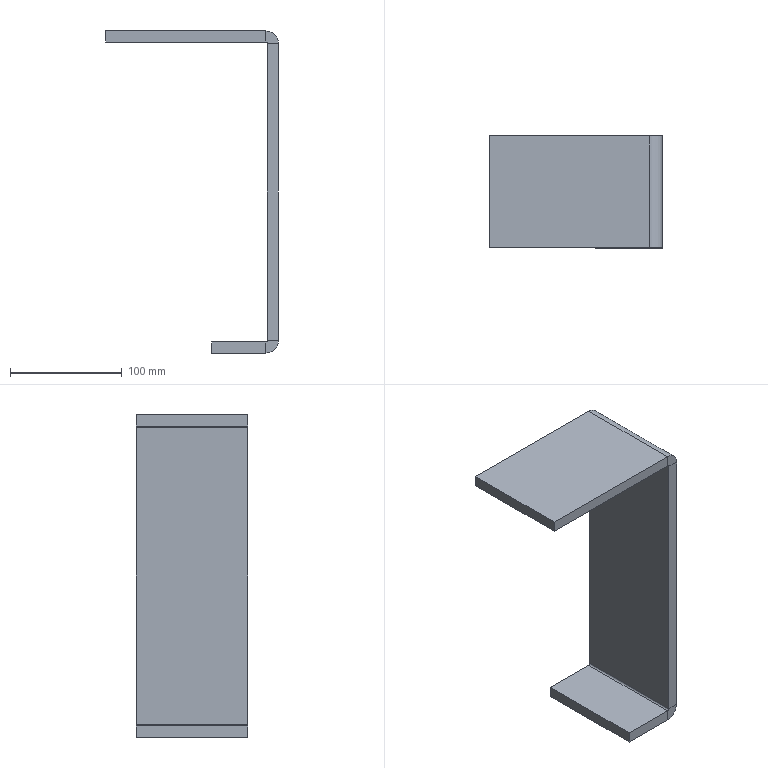Part | STEP file | A1 | 1 solid | 22 faces | box 155 x 100 x 289 mm | volume 478420 mm3 | plane 18 | cylinder 4 | commonest cylinder face diameters 3 x2 23 x2
STEP:
#1=CARTESIAN_POINT('',(0.,0.,0.));
#2=DIRECTION('',(0.,0.,1.));
#3=DIRECTION('',(1.,0.,0.));
#4=AXIS2_PLACEMENT_3D('',#1,#2,#3);
#5=CARTESIAN_POINT('',(50.,100.,267.5));
#6=VERTEX_POINT('',#5);
#7=CARTESIAN_POINT('',(60.,100.,267.5));
#8=VERTEX_POINT('',#7);
#9=CARTESIAN_POINT('',(50.,100.,267.5));
#10=DIRECTION('',(1.,0.,0.));
#11=VECTOR('',#10,1.);
#12=LINE('',#9,#11);
#13=CARTESIAN_POINT('',(60.,100.,279.));
#14=DIRECTION('',(0.,-1.,0.));
#15=DIRECTION('',(1.,0.,0.));
#16=AXIS2_PLACEMENT_3D('',#13,#14,#15);
#17=PLANE('',#16);
#18=CARTESIAN_POINT('',(-10.,-11.5));
#19=DIRECTION('',(1.,0.));
#20=VECTOR('',#19,1.);
#21=LINE('',#18,#20);
#22=(GEOMETRIC_REPRESENTATION_CONTEXT(2)PARAMETRIC_REPRESENTATION_CONTEXT()REPRESENTATION_CONTEXT('',''));
#23=DEFINITIONAL_REPRESENTATION('',(#21),#22);
#24=PCURVE('',#17,#23);
#25=CARTESIAN_POINT('',(48.5,100.,267.5));
#26=DIRECTION('',(0.,-1.,0.));
#27=DIRECTION('',(0.,0.,-1.));
#28=AXIS2_PLACEMENT_3D('',#25,#26,#27);
#29=PLANE('',#28);
#30=CARTESIAN_POINT('',(0.,1.5));
#31=DIRECTION('',(0.,1.));
#32=VECTOR('',#31,1.);
#33=LINE('',#30,#32);
#34=(GEOMETRIC_REPRESENTATION_CONTEXT(2)PARAMETRIC_REPRESENTATION_CONTEXT()REPRESENTATION_CONTEXT('',''));
#35=DEFINITIONAL_REPRESENTATION('',(#33),#34);
#36=PCURVE('',#29,#35);
#37=SURFACE_CURVE('',#12,(#24,#36),.PCURVE_S1.);
#38=EDGE_CURVE('',#6,#8,#37,.T.);
#39=ORIENTED_EDGE('',*,*,#38,.T.);
#40=CARTESIAN_POINT('',(60.,100.,1.5));
#41=VERTEX_POINT('',#40);
#42=CARTESIAN_POINT('',(60.,100.,0.));
#43=DIRECTION('',(0.,0.,1.));
#44=VECTOR('',#43,1.);
#45=LINE('',#42,#44);
#46=CARTESIAN_POINT('',(0.,-279.));
#47=DIRECTION('',(0.,1.));
#48=VECTOR('',#47,1.);
#49=LINE('',#46,#48);
#50=(GEOMETRIC_REPRESENTATION_CONTEXT(2)PARAMETRIC_REPRESENTATION_CONTEXT()REPRESENTATION_CONTEXT('',''));
#51=DEFINITIONAL_REPRESENTATION('',(#49),#50);
#52=PCURVE('',#17,#51);
#53=CARTESIAN_POINT('',(60.,0.,0.));
#54=DIRECTION('',(-1.,0.,0.));
#55=DIRECTION('',(0.,0.,1.));
#56=AXIS2_PLACEMENT_3D('',#53,#54,#55);
#57=PLANE('',#56);
#58=CARTESIAN_POINT('',(0.,100.));
#59=DIRECTION('',(1.,0.));
#60=VECTOR('',#59,1.);
#61=LINE('',#58,#60);
#62=(GEOMETRIC_REPRESENTATION_CONTEXT(2)PARAMETRIC_REPRESENTATION_CONTEXT()REPRESENTATION_CONTEXT('',''));
#63=DEFINITIONAL_REPRESENTATION('',(#61),#62);
#64=PCURVE('',#57,#63);
#65=SURFACE_CURVE('',#45,(#52,#64),.PCURVE_S1.);
#66=EDGE_CURVE('',#41,#8,#65,.T.);
#67=ORIENTED_EDGE('',*,*,#66,.F.);
#68=CARTESIAN_POINT('',(50.,100.,1.5));
#69=VERTEX_POINT('',#68);
#70=CARTESIAN_POINT('',(50.,100.,1.5));
#71=DIRECTION('',(1.,0.,0.));
#72=VECTOR('',#71,1.);
#73=LINE('',#70,#72);
#74=CARTESIAN_POINT('',(-10.,-277.5));
#75=DIRECTION('',(1.,0.));
#76=VECTOR('',#75,1.);
#77=LINE('',#74,#76);
#78=(GEOMETRIC_REPRESENTATION_CONTEXT(2)PARAMETRIC_REPRESENTATION_CONTEXT()REPRESENTATION_CONTEXT('',''));
#79=DEFINITIONAL_REPRESENTATION('',(#77),#78);
#80=PCURVE('',#17,#79);
#81=CARTESIAN_POINT('',(48.5,100.,1.5));
#82=DIRECTION('',(0.,-1.,0.));
#83=DIRECTION('',(0.,0.,-1.));
#84=AXIS2_PLACEMENT_3D('',#81,#82,#83);
#85=PLANE('',#84);
#86=CARTESIAN_POINT('',(0.,1.5));
#87=DIRECTION('',(0.,1.));
#88=VECTOR('',#87,1.);
#89=LINE('',#86,#88);
#90=(GEOMETRIC_REPRESENTATION_CONTEXT(2)PARAMETRIC_REPRESENTATION_CONTEXT()REPRESENTATION_CONTEXT('',''));
#91=DEFINITIONAL_REPRESENTATION('',(#89),#90);
#92=PCURVE('',#85,#91);
#93=SURFACE_CURVE('',#73,(#80,#92),.PCURVE_S1.);
#94=EDGE_CURVE('',#69,#41,#93,.T.);
#95=ORIENTED_EDGE('',*,*,#94,.F.);
#96=CARTESIAN_POINT('',(50.,100.,279.));
#97=DIRECTION('',(0.,0.,1.));
#98=VECTOR('',#97,1.);
#99=LINE('',#96,#98);
#100=CARTESIAN_POINT('',(-10.,0.));
#101=DIRECTION('',(0.,1.));
#102=VECTOR('',#101,1.);
#103=LINE('',#100,#102);
#104=(GEOMETRIC_REPRESENTATION_CONTEXT(2)PARAMETRIC_REPRESENTATION_CONTEXT()REPRESENTATION_CONTEXT('',''));
#105=DEFINITIONAL_REPRESENTATION('',(#103),#104);
#106=PCURVE('',#17,#105);
#107=CARTESIAN_POINT('',(50.,0.,0.));
#108=DIRECTION('',(-1.,0.,0.));
#109=DIRECTION('',(0.,0.,1.));
#110=AXIS2_PLACEMENT_3D('',#107,#108,#109);
#111=PLANE('',#110);
#112=CARTESIAN_POINT('',(279.,100.));
#113=DIRECTION('',(1.,0.));
#114=VECTOR('',#113,1.);
#115=LINE('',#112,#114);
#116=(GEOMETRIC_REPRESENTATION_CONTEXT(2)PARAMETRIC_REPRESENTATION_CONTEXT()REPRESENTATION_CONTEXT('',''));
#117=DEFINITIONAL_REPRESENTATION('',(#115),#116);
#118=PCURVE('',#111,#117);
#119=SURFACE_CURVE('',#99,(#106,#118),.PCURVE_S1.);
#120=EDGE_CURVE('',#69,#6,#119,.T.);
#121=ORIENTED_EDGE('',*,*,#120,.T.);
#122=EDGE_LOOP('',(#39,#67,#95,#121));
#123=FACE_BOUND('',#122,.T.);
#124=ADVANCED_FACE('',(#123),#17,.F.);
#125=CARTESIAN_POINT('',(50.,0.,267.5));
#126=VERTEX_POINT('',#125);
#127=CARTESIAN_POINT('',(60.,0.,267.5));
#128=VERTEX_POINT('',#127);
#129=CARTESIAN_POINT('',(50.,0.,267.5));
#130=DIRECTION('',(1.,0.,0.));
#131=VECTOR('',#130,1.);
#132=LINE('',#129,#131);
#133=CARTESIAN_POINT('',(60.,0.,0.));
#134=DIRECTION('',(0.,1.,0.));
#135=DIRECTION('',(-1.,0.,0.));
#136=AXIS2_PLACEMENT_3D('',#133,#134,#135);
#137=PLANE('',#136);
#138=CARTESIAN_POINT('',(10.,267.5));
#139=DIRECTION('',(-1.,0.));
#140=VECTOR('',#139,1.);
#141=LINE('',#138,#140);
#142=(GEOMETRIC_REPRESENTATION_CONTEXT(2)PARAMETRIC_REPRESENTATION_CONTEXT()REPRESENTATION_CONTEXT('',''));
#143=DEFINITIONAL_REPRESENTATION('',(#141),#142);
#144=PCURVE('',#137,#143);
#145=CARTESIAN_POINT('',(48.5,0.,267.5));
#146=DIRECTION('',(0.,-1.,0.));
#147=DIRECTION('',(0.,0.,-1.));
#148=AXIS2_PLACEMENT_3D('',#145,#146,#147);
#149=PLANE('',#148);
#150=CARTESIAN_POINT('',(0.,1.5));
#151=DIRECTION('',(0.,1.));
#152=VECTOR('',#151,1.);
#153=LINE('',#150,#152);
#154=(GEOMETRIC_REPRESENTATION_CONTEXT(2)PARAMETRIC_REPRESENTATION_CONTEXT()REPRESENTATION_CONTEXT('',''));
#155=DEFINITIONAL_REPRESENTATION('',(#153),#154);
#156=PCURVE('',#149,#155);
#157=SURFACE_CURVE('',#132,(#144,#156),.PCURVE_S1.);
#158=EDGE_CURVE('',#126,#128,#157,.T.);
#159=ORIENTED_EDGE('',*,*,#158,.F.);
#160=CARTESIAN_POINT('',(50.,0.,1.5));
#161=VERTEX_POINT('',#160);
#162=CARTESIAN_POINT('',(50.,0.,0.));
#163=DIRECTION('',(0.,0.,-1.));
#164=VECTOR('',#163,1.);
#165=LINE('',#162,#164);
#166=CARTESIAN_POINT('',(10.,0.));
#167=DIRECTION('',(0.,-1.));
#168=VECTOR('',#167,1.);
#169=LINE('',#166,#168);
#170=(GEOMETRIC_REPRESENTATION_CONTEXT(2)PARAMETRIC_REPRESENTATION_CONTEXT()REPRESENTATION_CONTEXT('',''));
#171=DEFINITIONAL_REPRESENTATION('',(#169),#170);
#172=PCURVE('',#137,#171);
#173=CARTESIAN_POINT('',(0.,0.));
#174=DIRECTION('',(-1.,0.));
#175=VECTOR('',#174,1.);
#176=LINE('',#173,#175);
#177=(GEOMETRIC_REPRESENTATION_CONTEXT(2)PARAMETRIC_REPRESENTATION_CONTEXT()REPRESENTATION_CONTEXT('',''));
#178=DEFINITIONAL_REPRESENTATION('',(#176),#177);
#179=PCURVE('',#111,#178);
#180=SURFACE_CURVE('',#165,(#172,#179),.PCURVE_S1.);
#181=EDGE_CURVE('',#126,#161,#180,.T.);
#182=ORIENTED_EDGE('',*,*,#181,.T.);
#183=CARTESIAN_POINT('',(60.,0.,1.5));
#184=VERTEX_POINT('',#183);
#185=CARTESIAN_POINT('',(60.,0.,1.5));
#186=DIRECTION('',(1.,0.,0.));
#187=VECTOR('',#186,1.);
#188=LINE('',#185,#187);
#189=CARTESIAN_POINT('',(0.,1.5));
#190=DIRECTION('',(-1.,0.));
#191=VECTOR('',#190,1.);
#192=LINE('',#189,#191);
#193=(GEOMETRIC_REPRESENTATION_CONTEXT(2)PARAMETRIC_REPRESENTATION_CONTEXT()REPRESENTATION_CONTEXT('',''));
#194=DEFINITIONAL_REPRESENTATION('',(#192),#193);
#195=PCURVE('',#137,#194);
#196=CARTESIAN_POINT('',(48.5,0.,1.5));
#197=DIRECTION('',(0.,-1.,0.));
#198=DIRECTION('',(0.,0.,-1.));
#199=AXIS2_PLACEMENT_3D('',#196,#197,#198);
#200=PLANE('',#199);
#201=CARTESIAN_POINT('',(0.,11.5));
#202=DIRECTION('',(0.,1.));
#203=VECTOR('',#202,1.);
#204=LINE('',#201,#203);
#205=(GEOMETRIC_REPRESENTATION_CONTEXT(2)PARAMETRIC_REPRESENTATION_CONTEXT()REPRESENTATION_CONTEXT('',''));
#206=DEFINITIONAL_REPRESENTATION('',(#204),#205);
#207=PCURVE('',#200,#206);
#208=SURFACE_CURVE('',#188,(#195,#207),.PCURVE_S1.);
#209=EDGE_CURVE('',#161,#184,#208,.T.);
#210=ORIENTED_EDGE('',*,*,#209,.T.);
#211=CARTESIAN_POINT('',(60.,0.,0.));
#212=DIRECTION('',(0.,0.,-1.));
#213=VECTOR('',#212,1.);
#214=LINE('',#211,#213);
#215=CARTESIAN_POINT('',(0.,0.));
#216=DIRECTION('',(0.,-1.));
#217=VECTOR('',#216,1.);
#218=LINE('',#215,#217);
#219=(GEOMETRIC_REPRESENTATION_CONTEXT(2)PARAMETRIC_REPRESENTATION_CONTEXT()REPRESENTATION_CONTEXT('',''));
#220=DEFINITIONAL_REPRESENTATION('',(#218),#219);
#221=PCURVE('',#137,#220);
#222=CARTESIAN_POINT('',(0.,0.));
#223=DIRECTION('',(-1.,0.));
#224=VECTOR('',#223,1.);
#225=LINE('',#222,#224);
#226=(GEOMETRIC_REPRESENTATION_CONTEXT(2)PARAMETRIC_REPRESENTATION_CONTEXT()REPRESENTATION_CONTEXT('',''));
#227=DEFINITIONAL_REPRESENTATION('',(#225),#226);
#228=PCURVE('',#57,#227);
#229=SURFACE_CURVE('',#214,(#221,#228),.PCURVE_S1.);
#230=EDGE_CURVE('',#128,#184,#229,.T.);
#231=ORIENTED_EDGE('',*,*,#230,.F.);
#232=EDGE_LOOP('',(#159,#182,#210,#231));
#233=FACE_BOUND('',#232,.T.);
#234=ADVANCED_FACE('',(#233),#137,.F.);
#235=CARTESIAN_POINT('',(60.,100.,267.5));
#236=DIRECTION('',(0.,-1.,0.));
#237=VECTOR('',#236,1.);
#238=LINE('',#235,#237);
#239=CARTESIAN_POINT('',(267.5,100.));
#240=DIRECTION('',(0.,-1.));
#241=VECTOR('',#240,1.);
#242=LINE('',#239,#241);
#243=(GEOMETRIC_REPRESENTATION_CONTEXT(2)PARAMETRIC_REPRESENTATION_CONTEXT()REPRESENTATION_CONTEXT('',''));
#244=DEFINITIONAL_REPRESENTATION('',(#242),#243);
#245=PCURVE('',#57,#244);
#246=CARTESIAN_POINT('',(48.5,100.,267.5));
#247=DIRECTION('',(0.,1.,0.));
#248=DIRECTION('',(0.,0.,1.));
#249=AXIS2_PLACEMENT_3D('',#246,#247,#248);
#250=CYLINDRICAL_SURFACE('',#249,11.5);
#251=CARTESIAN_POINT('',(1.571,0.));
#252=DIRECTION('',(0.,-1.));
#253=VECTOR('',#252,1.);
#254=LINE('',#251,#253);
#255=(GEOMETRIC_REPRESENTATION_CONTEXT(2)PARAMETRIC_REPRESENTATION_CONTEXT()REPRESENTATION_CONTEXT('',''));
#256=DEFINITIONAL_REPRESENTATION('',(#254),#255);
#257=PCURVE('',#250,#256);
#258=SURFACE_CURVE('',#238,(#245,#257),.PCURVE_S1.);
#259=EDGE_CURVE('',#8,#128,#258,.T.);
#260=ORIENTED_EDGE('',*,*,#259,.T.);
#261=ORIENTED_EDGE('',*,*,#230,.T.);
#262=CARTESIAN_POINT('',(60.,0.,1.5));
#263=DIRECTION('',(0.,-1.,0.));
#264=VECTOR('',#263,1.);
#265=LINE('',#262,#264);
#266=CARTESIAN_POINT('',(1.5,0.));
#267=DIRECTION('',(0.,-1.));
#268=VECTOR('',#267,1.);
#269=LINE('',#266,#268);
#270=(GEOMETRIC_REPRESENTATION_CONTEXT(2)PARAMETRIC_REPRESENTATION_CONTEXT()REPRESENTATION_CONTEXT('',''));
#271=DEFINITIONAL_REPRESENTATION('',(#269),#270);
#272=PCURVE('',#57,#271);
#273=CARTESIAN_POINT('',(48.5,100.,1.5));
#274=DIRECTION('',(0.,1.,0.));
#275=DIRECTION('',(1.,0.,0.));
#276=AXIS2_PLACEMENT_3D('',#273,#274,#275);
#277=CYLINDRICAL_SURFACE('',#276,11.5);
#278=CARTESIAN_POINT('',(0.,-100.));
#279=DIRECTION('',(0.,-1.));
#280=VECTOR('',#279,1.);
#281=LINE('',#278,#280);
#282=(GEOMETRIC_REPRESENTATION_CONTEXT(2)PARAMETRIC_REPRESENTATION_CONTEXT()REPRESENTATION_CONTEXT('',''));
#283=DEFINITIONAL_REPRESENTATION('',(#281),#282);
#284=PCURVE('',#277,#283);
#285=SURFACE_CURVE('',#265,(#272,#284),.PCURVE_S1.);
#286=EDGE_CURVE('',#41,#184,#285,.T.);
#287=ORIENTED_EDGE('',*,*,#286,.F.);
#288=ORIENTED_EDGE('',*,*,#66,.T.);
#289=EDGE_LOOP('',(#260,#261,#287,#288));
#290=FACE_BOUND('',#289,.T.);
#291=ADVANCED_FACE('',(#290),#57,.F.);
#292=ORIENTED_EDGE('',*,*,#181,.F.);
#293=CARTESIAN_POINT('',(50.,100.,267.5));
#294=DIRECTION('',(0.,-1.,0.));
#295=VECTOR('',#294,1.);
#296=LINE('',#293,#295);
#297=CARTESIAN_POINT('',(267.5,100.));
#298=DIRECTION('',(0.,-1.));
#299=VECTOR('',#298,1.);
#300=LINE('',#297,#299);
#301=(GEOMETRIC_REPRESENTATION_CONTEXT(2)PARAMETRIC_REPRESENTATION_CONTEXT()REPRESENTATION_CONTEXT('',''));
#302=DEFINITIONAL_REPRESENTATION('',(#300),#301);
#303=PCURVE('',#111,#302);
#304=CARTESIAN_POINT('',(48.5,100.,267.5));
#305=DIRECTION('',(0.,1.,0.));
#306=DIRECTION('',(0.,0.,1.));
#307=AXIS2_PLACEMENT_3D('',#304,#305,#306);
#308=CYLINDRICAL_SURFACE('',#307,1.5);
#309=CARTESIAN_POINT('',(1.571,0.));
#310=DIRECTION('',(0.,-1.));
#311=VECTOR('',#310,1.);
#312=LINE('',#309,#311);
#313=(GEOMETRIC_REPRESENTATION_CONTEXT(2)PARAMETRIC_REPRESENTATION_CONTEXT()REPRESENTATION_CONTEXT('',''));
#314=DEFINITIONAL_REPRESENTATION('',(#312),#313);
#315=PCURVE('',#308,#314);
#316=SURFACE_CURVE('',#296,(#303,#315),.PCURVE_S1.);
#317=EDGE_CURVE('',#6,#126,#316,.T.);
#318=ORIENTED_EDGE('',*,*,#317,.F.);
#319=ORIENTED_EDGE('',*,*,#120,.F.);
#320=CARTESIAN_POINT('',(50.,0.,1.5));
#321=DIRECTION('',(0.,1.,0.));
#322=VECTOR('',#321,1.);
#323=LINE('',#320,#322);
#324=CARTESIAN_POINT('',(1.5,0.));
#325=DIRECTION('',(0.,1.));
#326=VECTOR('',#325,1.);
#327=LINE('',#324,#326);
#328=(GEOMETRIC_REPRESENTATION_CONTEXT(2)PARAMETRIC_REPRESENTATION_CONTEXT()REPRESENTATION_CONTEXT('',''));
#329=DEFINITIONAL_REPRESENTATION('',(#327),#328);
#330=PCURVE('',#111,#329);
#331=CARTESIAN_POINT('',(48.5,100.,1.5));
#332=DIRECTION('',(0.,1.,0.));
#333=DIRECTION('',(1.,0.,0.));
#334=AXIS2_PLACEMENT_3D('',#331,#332,#333);
#335=CYLINDRICAL_SURFACE('',#334,1.5);
#336=CARTESIAN_POINT('',(0.,-100.));
#337=DIRECTION('',(0.,1.));
#338=VECTOR('',#337,1.);
#339=LINE('',#336,#338);
#340=(GEOMETRIC_REPRESENTATION_CONTEXT(2)PARAMETRIC_REPRESENTATION_CONTEXT()REPRESENTATION_CONTEXT('',''));
#341=DEFINITIONAL_REPRESENTATION('',(#339),#340);
#342=PCURVE('',#335,#341);
#343=SURFACE_CURVE('',#323,(#330,#342),.PCURVE_S1.);
#344=EDGE_CURVE('',#161,#69,#343,.T.);
#345=ORIENTED_EDGE('',*,*,#344,.F.);
#346=EDGE_LOOP('',(#292,#318,#319,#345));
#347=FACE_BOUND('',#346,.T.);
#348=ADVANCED_FACE('',(#347),#111,.T.);
#349=CARTESIAN_POINT('',(48.5,100.,0.));
#350=VERTEX_POINT('',#349);
#351=CARTESIAN_POINT('',(0.,100.,0.));
#352=VERTEX_POINT('',#351);
#353=CARTESIAN_POINT('',(0.,100.,0.));
#354=DIRECTION('',(-1.,0.,0.));
#355=VECTOR('',#354,1.);
#356=LINE('',#353,#355);
#357=CARTESIAN_POINT('',(0.,100.,-10.));
#358=DIRECTION('',(0.,1.,0.));
#359=DIRECTION('',(-1.,0.,0.));
#360=AXIS2_PLACEMENT_3D('',#357,#358,#359);
#361=PLANE('',#360);
#362=CARTESIAN_POINT('',(0.,10.));
#363=DIRECTION('',(1.,0.));
#364=VECTOR('',#363,1.);
#365=LINE('',#362,#364);
#366=(GEOMETRIC_REPRESENTATION_CONTEXT(2)PARAMETRIC_REPRESENTATION_CONTEXT()REPRESENTATION_CONTEXT('',''));
#367=DEFINITIONAL_REPRESENTATION('',(#365),#366);
#368=PCURVE('',#361,#367);
#369=CARTESIAN_POINT('',(0.,0.,0.));
#370=DIRECTION('',(0.,0.,1.));
#371=DIRECTION('',(1.,0.,0.));
#372=AXIS2_PLACEMENT_3D('',#369,#370,#371);
#373=PLANE('',#372);
#374=CARTESIAN_POINT('',(0.,100.));
#375=DIRECTION('',(-1.,0.));
#376=VECTOR('',#375,1.);
#377=LINE('',#374,#376);
#378=(GEOMETRIC_REPRESENTATION_CONTEXT(2)PARAMETRIC_REPRESENTATION_CONTEXT()REPRESENTATION_CONTEXT('',''));
#379=DEFINITIONAL_REPRESENTATION('',(#377),#378);
#380=PCURVE('',#373,#379);
#381=SURFACE_CURVE('',#356,(#368,#380),.PCURVE_S1.);
#382=EDGE_CURVE('',#350,#352,#381,.T.);
#383=ORIENTED_EDGE('',*,*,#382,.F.);
#384=CARTESIAN_POINT('',(48.5,100.,-10.));
#385=VERTEX_POINT('',#384);
#386=CARTESIAN_POINT('',(48.5,100.,0.));
#387=DIRECTION('',(0.,0.,-1.));
#388=VECTOR('',#387,1.);
#389=LINE('',#386,#388);
#390=CARTESIAN_POINT('',(-48.5,10.));
#391=DIRECTION('',(0.,-1.));
#392=VECTOR('',#391,1.);
#393=LINE('',#390,#392);
#394=(GEOMETRIC_REPRESENTATION_CONTEXT(2)PARAMETRIC_REPRESENTATION_CONTEXT()REPRESENTATION_CONTEXT('',''));
#395=DEFINITIONAL_REPRESENTATION('',(#393),#394);
#396=PCURVE('',#361,#395);
#397=CARTESIAN_POINT('',(1.5,0.));
#398=DIRECTION('',(1.,0.));
#399=VECTOR('',#398,1.);
#400=LINE('',#397,#399);
#401=(GEOMETRIC_REPRESENTATION_CONTEXT(2)PARAMETRIC_REPRESENTATION_CONTEXT()REPRESENTATION_CONTEXT('',''));
#402=DEFINITIONAL_REPRESENTATION('',(#400),#401);
#403=PCURVE('',#85,#402);
#404=SURFACE_CURVE('',#389,(#396,#403),.PCURVE_S1.);
#405=EDGE_CURVE('',#350,#385,#404,.T.);
#406=ORIENTED_EDGE('',*,*,#405,.T.);
#407=CARTESIAN_POINT('',(0.,100.,-10.));
#408=VERTEX_POINT('',#407);
#409=CARTESIAN_POINT('',(0.,100.,-10.));
#410=DIRECTION('',(-1.,0.,0.));
#411=VECTOR('',#410,1.);
#412=LINE('',#409,#411);
#413=CARTESIAN_POINT('',(0.,0.));
#414=DIRECTION('',(1.,0.));
#415=VECTOR('',#414,1.);
#416=LINE('',#413,#415);
#417=(GEOMETRIC_REPRESENTATION_CONTEXT(2)PARAMETRIC_REPRESENTATION_CONTEXT()REPRESENTATION_CONTEXT('',''));
#418=DEFINITIONAL_REPRESENTATION('',(#416),#417);
#419=PCURVE('',#361,#418);
#420=CARTESIAN_POINT('',(0.,0.,-10.));
#421=DIRECTION('',(0.,0.,1.));
#422=DIRECTION('',(1.,0.,0.));
#423=AXIS2_PLACEMENT_3D('',#420,#421,#422);
#424=PLANE('',#423);
#425=CARTESIAN_POINT('',(0.,100.));
#426=DIRECTION('',(-1.,0.));
#427=VECTOR('',#426,1.);
#428=LINE('',#425,#427);
#429=(GEOMETRIC_REPRESENTATION_CONTEXT(2)PARAMETRIC_REPRESENTATION_CONTEXT()REPRESENTATION_CONTEXT('',''));
#430=DEFINITIONAL_REPRESENTATION('',(#428),#429);
#431=PCURVE('',#424,#430);
#432=SURFACE_CURVE('',#412,(#419,#431),.PCURVE_S1.);
#433=EDGE_CURVE('',#385,#408,#432,.T.);
#434=ORIENTED_EDGE('',*,*,#433,.T.);
#435=CARTESIAN_POINT('',(0.,100.,-10.));
#436=DIRECTION('',(0.,0.,1.));
#437=VECTOR('',#436,1.);
#438=LINE('',#435,#437);
#439=CARTESIAN_POINT('',(0.,0.));
#440=DIRECTION('',(0.,1.));
#441=VECTOR('',#440,1.);
#442=LINE('',#439,#441);
#443=(GEOMETRIC_REPRESENTATION_CONTEXT(2)PARAMETRIC_REPRESENTATION_CONTEXT()REPRESENTATION_CONTEXT('',''));
#444=DEFINITIONAL_REPRESENTATION('',(#442),#443);
#445=PCURVE('',#361,#444);
#446=CARTESIAN_POINT('',(0.,100.,-10.));
#447=DIRECTION('',(-1.,0.,0.));
#448=DIRECTION('',(0.,-1.,0.));
#449=AXIS2_PLACEMENT_3D('',#446,#447,#448);
#450=PLANE('',#449);
#451=CARTESIAN_POINT('',(0.,0.));
#452=DIRECTION('',(0.,1.));
#453=VECTOR('',#452,1.);
#454=LINE('',#451,#453);
#455=(GEOMETRIC_REPRESENTATION_CONTEXT(2)PARAMETRIC_REPRESENTATION_CONTEXT()REPRESENTATION_CONTEXT('',''));
#456=DEFINITIONAL_REPRESENTATION('',(#454),#455);
#457=PCURVE('',#450,#456);
#458=SURFACE_CURVE('',#438,(#445,#457),.PCURVE_S1.);
#459=EDGE_CURVE('',#408,#352,#458,.T.);
#460=ORIENTED_EDGE('',*,*,#459,.T.);
#461=EDGE_LOOP('',(#383,#406,#434,#460));
#462=FACE_BOUND('',#461,.T.);
#463=ADVANCED_FACE('',(#462),#361,.T.);
#464=CARTESIAN_POINT('',(48.5,0.,-10.));
#465=VERTEX_POINT('',#464);
#466=CARTESIAN_POINT('',(48.5,100.,-10.));
#467=DIRECTION('',(0.,-1.,0.));
#468=VECTOR('',#467,1.);
#469=LINE('',#466,#468);
#470=CARTESIAN_POINT('',(48.5,100.));
#471=DIRECTION('',(0.,-1.));
#472=VECTOR('',#471,1.);
#473=LINE('',#470,#472);
#474=(GEOMETRIC_REPRESENTATION_CONTEXT(2)PARAMETRIC_REPRESENTATION_CONTEXT()REPRESENTATION_CONTEXT('',''));
#475=DEFINITIONAL_REPRESENTATION('',(#473),#474);
#476=PCURVE('',#424,#475);
#477=CARTESIAN_POINT('',(1.571,0.));
#478=DIRECTION('',(0.,-1.));
#479=VECTOR('',#478,1.);
#480=LINE('',#477,#479);
#481=(GEOMETRIC_REPRESENTATION_CONTEXT(2)PARAMETRIC_REPRESENTATION_CONTEXT()REPRESENTATION_CONTEXT('',''));
#482=DEFINITIONAL_REPRESENTATION('',(#480),#481);
#483=PCURVE('',#277,#482);
#484=SURFACE_CURVE('',#469,(#476,#483),.PCURVE_S1.);
#485=EDGE_CURVE('',#385,#465,#484,.T.);
#486=ORIENTED_EDGE('',*,*,#485,.T.);
#487=CARTESIAN_POINT('',(0.,0.,-10.));
#488=VERTEX_POINT('',#487);
#489=CARTESIAN_POINT('',(0.,0.,-10.));
#490=DIRECTION('',(1.,0.,0.));
#491=VECTOR('',#490,1.);
#492=LINE('',#489,#491);
#493=CARTESIAN_POINT('',(0.,0.));
#494=DIRECTION('',(1.,0.));
#495=VECTOR('',#494,1.);
#496=LINE('',#493,#495);
#497=(GEOMETRIC_REPRESENTATION_CONTEXT(2)PARAMETRIC_REPRESENTATION_CONTEXT()REPRESENTATION_CONTEXT('',''));
#498=DEFINITIONAL_REPRESENTATION('',(#496),#497);
#499=PCURVE('',#424,#498);
#500=CARTESIAN_POINT('',(0.,0.,-10.));
#501=DIRECTION('',(0.,-1.,0.));
#502=DIRECTION('',(1.,0.,0.));
#503=AXIS2_PLACEMENT_3D('',#500,#501,#502);
#504=PLANE('',#503);
#505=CARTESIAN_POINT('',(0.,0.));
#506=DIRECTION('',(1.,0.));
#507=VECTOR('',#506,1.);
#508=LINE('',#505,#507);
#509=(GEOMETRIC_REPRESENTATION_CONTEXT(2)PARAMETRIC_REPRESENTATION_CONTEXT()REPRESENTATION_CONTEXT('',''));
#510=DEFINITIONAL_REPRESENTATION('',(#508),#509);
#511=PCURVE('',#504,#510);
#512=SURFACE_CURVE('',#492,(#499,#511),.PCURVE_S1.);
#513=EDGE_CURVE('',#488,#465,#512,.T.);
#514=ORIENTED_EDGE('',*,*,#513,.F.);
#515=CARTESIAN_POINT('',(0.,100.,-10.));
#516=DIRECTION('',(0.,-1.,0.));
#517=VECTOR('',#516,1.);
#518=LINE('',#515,#517);
#519=CARTESIAN_POINT('',(0.,100.));
#520=DIRECTION('',(0.,-1.));
#521=VECTOR('',#520,1.);
#522=LINE('',#519,#521);
#523=(GEOMETRIC_REPRESENTATION_CONTEXT(2)PARAMETRIC_REPRESENTATION_CONTEXT()REPRESENTATION_CONTEXT('',''));
#524=DEFINITIONAL_REPRESENTATION('',(#522),#523);
#525=PCURVE('',#424,#524);
#526=CARTESIAN_POINT('',(0.,0.));
#527=DIRECTION('',(1.,0.));
#528=VECTOR('',#527,1.);
#529=LINE('',#526,#528);
#530=(GEOMETRIC_REPRESENTATION_CONTEXT(2)PARAMETRIC_REPRESENTATION_CONTEXT()REPRESENTATION_CONTEXT('',''));
#531=DEFINITIONAL_REPRESENTATION('',(#529),#530);
#532=PCURVE('',#450,#531);
#533=SURFACE_CURVE('',#518,(#525,#532),.PCURVE_S1.);
#534=EDGE_CURVE('',#408,#488,#533,.T.);
#535=ORIENTED_EDGE('',*,*,#534,.F.);
#536=ORIENTED_EDGE('',*,*,#433,.F.);
#537=EDGE_LOOP('',(#486,#514,#535,#536));
#538=FACE_BOUND('',#537,.T.);
#539=ADVANCED_FACE('',(#538),#424,.F.);
#540=CARTESIAN_POINT('',(0.,0.,0.));
#541=VERTEX_POINT('',#540);
#542=CARTESIAN_POINT('',(48.5,0.,0.));
#543=VERTEX_POINT('',#542);
#544=CARTESIAN_POINT('',(0.,0.,0.));
#545=DIRECTION('',(1.,0.,0.));
#546=VECTOR('',#545,1.);
#547=LINE('',#544,#546);
#548=CARTESIAN_POINT('',(0.,0.));
#549=DIRECTION('',(1.,0.));
#550=VECTOR('',#549,1.);
#551=LINE('',#548,#550);
#552=(GEOMETRIC_REPRESENTATION_CONTEXT(2)PARAMETRIC_REPRESENTATION_CONTEXT()REPRESENTATION_CONTEXT('',''));
#553=DEFINITIONAL_REPRESENTATION('',(#551),#552);
#554=PCURVE('',#373,#553);
#555=CARTESIAN_POINT('',(0.,10.));
#556=DIRECTION('',(1.,0.));
#557=VECTOR('',#556,1.);
#558=LINE('',#555,#557);
#559=(GEOMETRIC_REPRESENTATION_CONTEXT(2)PARAMETRIC_REPRESENTATION_CONTEXT()REPRESENTATION_CONTEXT('',''));
#560=DEFINITIONAL_REPRESENTATION('',(#558),#559);
#561=PCURVE('',#504,#560);
#562=SURFACE_CURVE('',#547,(#554,#561),.PCURVE_S1.);
#563=EDGE_CURVE('',#541,#543,#562,.T.);
#564=ORIENTED_EDGE('',*,*,#563,.T.);
#565=CARTESIAN_POINT('',(48.5,100.,0.));
#566=DIRECTION('',(0.,-1.,0.));
#567=VECTOR('',#566,1.);
#568=LINE('',#565,#567);
#569=CARTESIAN_POINT('',(48.5,100.));
#570=DIRECTION('',(0.,-1.));
#571=VECTOR('',#570,1.);
#572=LINE('',#569,#571);
#573=(GEOMETRIC_REPRESENTATION_CONTEXT(2)PARAMETRIC_REPRESENTATION_CONTEXT()REPRESENTATION_CONTEXT('',''));
#574=DEFINITIONAL_REPRESENTATION('',(#572),#573);
#575=PCURVE('',#373,#574);
#576=CARTESIAN_POINT('',(1.571,0.));
#577=DIRECTION('',(0.,-1.));
#578=VECTOR('',#577,1.);
#579=LINE('',#576,#578);
#580=(GEOMETRIC_REPRESENTATION_CONTEXT(2)PARAMETRIC_REPRESENTATION_CONTEXT()REPRESENTATION_CONTEXT('',''));
#581=DEFINITIONAL_REPRESENTATION('',(#579),#580);
#582=PCURVE('',#335,#581);
#583=SURFACE_CURVE('',#568,(#575,#582),.PCURVE_S1.);
#584=EDGE_CURVE('',#350,#543,#583,.T.);
#585=ORIENTED_EDGE('',*,*,#584,.F.);
#586=ORIENTED_EDGE('',*,*,#382,.T.);
#587=CARTESIAN_POINT('',(0.,100.,0.));
#588=DIRECTION('',(0.,-1.,0.));
#589=VECTOR('',#588,1.);
#590=LINE('',#587,#589);
#591=CARTESIAN_POINT('',(0.,100.));
#592=DIRECTION('',(0.,-1.));
#593=VECTOR('',#592,1.);
#594=LINE('',#591,#593);
#595=(GEOMETRIC_REPRESENTATION_CONTEXT(2)PARAMETRIC_REPRESENTATION_CONTEXT()REPRESENTATION_CONTEXT('',''));
#596=DEFINITIONAL_REPRESENTATION('',(#594),#595);
#597=PCURVE('',#373,#596);
#598=CARTESIAN_POINT('',(0.,10.));
#599=DIRECTION('',(1.,0.));
#600=VECTOR('',#599,1.);
#601=LINE('',#598,#600);
#602=(GEOMETRIC_REPRESENTATION_CONTEXT(2)PARAMETRIC_REPRESENTATION_CONTEXT()REPRESENTATION_CONTEXT('',''));
#603=DEFINITIONAL_REPRESENTATION('',(#601),#602);
#604=PCURVE('',#450,#603);
#605=SURFACE_CURVE('',#590,(#597,#604),.PCURVE_S1.);
#606=EDGE_CURVE('',#352,#541,#605,.T.);
#607=ORIENTED_EDGE('',*,*,#606,.T.);
#608=EDGE_LOOP('',(#564,#585,#586,#607));
#609=FACE_BOUND('',#608,.T.);
#610=ADVANCED_FACE('',(#609),#373,.T.);
#611=ORIENTED_EDGE('',*,*,#606,.F.);
#612=ORIENTED_EDGE('',*,*,#459,.F.);
#613=ORIENTED_EDGE('',*,*,#534,.T.);
#614=CARTESIAN_POINT('',(0.,0.,-10.));
#615=DIRECTION('',(0.,0.,1.));
#616=VECTOR('',#615,1.);
#617=LINE('',#614,#616);
#618=CARTESIAN_POINT('',(100.,0.));
#619=DIRECTION('',(0.,1.));
#620=VECTOR('',#619,1.);
#621=LINE('',#618,#620);
#622=(GEOMETRIC_REPRESENTATION_CONTEXT(2)PARAMETRIC_REPRESENTATION_CONTEXT()REPRESENTATION_CONTEXT('',''));
#623=DEFINITIONAL_REPRESENTATION('',(#621),#622);
#624=PCURVE('',#450,#623);
#625=CARTESIAN_POINT('',(0.,0.));
#626=DIRECTION('',(0.,1.));
#627=VECTOR('',#626,1.);
#628=LINE('',#625,#627);
#629=(GEOMETRIC_REPRESENTATION_CONTEXT(2)PARAMETRIC_REPRESENTATION_CONTEXT()REPRESENTATION_CONTEXT('',''));
#630=DEFINITIONAL_REPRESENTATION('',(#628),#629);
#631=PCURVE('',#504,#630);
#632=SURFACE_CURVE('',#617,(#624,#631),.PCURVE_S1.);
#633=EDGE_CURVE('',#488,#541,#632,.T.);
#634=ORIENTED_EDGE('',*,*,#633,.T.);
#635=EDGE_LOOP('',(#611,#612,#613,#634));
#636=FACE_BOUND('',#635,.T.);
#637=ADVANCED_FACE('',(#636),#450,.T.);
#638=CARTESIAN_POINT('',(48.5,0.,0.));
#639=DIRECTION('',(0.,0.,-1.));
#640=VECTOR('',#639,1.);
#641=LINE('',#638,#640);
#642=CARTESIAN_POINT('',(48.5,10.));
#643=DIRECTION('',(0.,-1.));
#644=VECTOR('',#643,1.);
#645=LINE('',#642,#644);
#646=(GEOMETRIC_REPRESENTATION_CONTEXT(2)PARAMETRIC_REPRESENTATION_CONTEXT()REPRESENTATION_CONTEXT('',''));
#647=DEFINITIONAL_REPRESENTATION('',(#645),#646);
#648=PCURVE('',#504,#647);
#649=CARTESIAN_POINT('',(1.5,0.));
#650=DIRECTION('',(1.,0.));
#651=VECTOR('',#650,1.);
#652=LINE('',#649,#651);
#653=(GEOMETRIC_REPRESENTATION_CONTEXT(2)PARAMETRIC_REPRESENTATION_CONTEXT()REPRESENTATION_CONTEXT('',''));
#654=DEFINITIONAL_REPRESENTATION('',(#652),#653);
#655=PCURVE('',#200,#654);
#656=SURFACE_CURVE('',#641,(#648,#655),.PCURVE_S1.);
#657=EDGE_CURVE('',#543,#465,#656,.T.);
#658=ORIENTED_EDGE('',*,*,#657,.F.);
#659=ORIENTED_EDGE('',*,*,#563,.F.);
#660=ORIENTED_EDGE('',*,*,#633,.F.);
#661=ORIENTED_EDGE('',*,*,#513,.T.);
#662=EDGE_LOOP('',(#658,#659,#660,#661));
#663=FACE_BOUND('',#662,.T.);
#664=ADVANCED_FACE('',(#663),#504,.T.);
#665=ORIENTED_EDGE('',*,*,#209,.F.);
#666=CARTESIAN_POINT('',(48.5,0.,1.5));
#667=DIRECTION('',(0.,-1.,0.));
#668=DIRECTION('',(0.,0.,1.));
#669=AXIS2_PLACEMENT_3D('',#666,#667,#668);
#670=CIRCLE('',#669,1.5);
#671=CARTESIAN_POINT('',(0.,0.));
#672=DIRECTION('',(-1.,0.));
#673=AXIS2_PLACEMENT_2D('',#671,#672);
#674=CIRCLE('',#673,1.5);
#675=(GEOMETRIC_REPRESENTATION_CONTEXT(2)PARAMETRIC_REPRESENTATION_CONTEXT()REPRESENTATION_CONTEXT('',''));
#676=DEFINITIONAL_REPRESENTATION('',(#674),#675);
#677=PCURVE('',#200,#676);
#678=CARTESIAN_POINT('',(4.712,-100.));
#679=DIRECTION('',(-1.,0.));
#680=VECTOR('',#679,1.);
#681=LINE('',#678,#680);
#682=(GEOMETRIC_REPRESENTATION_CONTEXT(2)PARAMETRIC_REPRESENTATION_CONTEXT()REPRESENTATION_CONTEXT('',''));
#683=DEFINITIONAL_REPRESENTATION('',(#681),#682);
#684=PCURVE('',#335,#683);
#685=SURFACE_CURVE('',#670,(#677,#684),.PCURVE_S1.);
#686=EDGE_CURVE('',#543,#161,#685,.T.);
#687=ORIENTED_EDGE('',*,*,#686,.F.);
#688=ORIENTED_EDGE('',*,*,#657,.T.);
#689=CARTESIAN_POINT('',(48.5,0.,1.5));
#690=DIRECTION('',(0.,-1.,0.));
#691=DIRECTION('',(0.,0.,1.));
#692=AXIS2_PLACEMENT_3D('',#689,#690,#691);
#693=CIRCLE('',#692,11.5);
#694=CARTESIAN_POINT('',(0.,0.));
#695=DIRECTION('',(-1.,0.));
#696=AXIS2_PLACEMENT_2D('',#694,#695);
#697=CIRCLE('',#696,11.5);
#698=(GEOMETRIC_REPRESENTATION_CONTEXT(2)PARAMETRIC_REPRESENTATION_CONTEXT()REPRESENTATION_CONTEXT('',''));
#699=DEFINITIONAL_REPRESENTATION('',(#697),#698);
#700=PCURVE('',#200,#699);
#701=CARTESIAN_POINT('',(4.712,-100.));
#702=DIRECTION('',(-1.,0.));
#703=VECTOR('',#702,1.);
#704=LINE('',#701,#703);
#705=(GEOMETRIC_REPRESENTATION_CONTEXT(2)PARAMETRIC_REPRESENTATION_CONTEXT()REPRESENTATION_CONTEXT('',''));
#706=DEFINITIONAL_REPRESENTATION('',(#704),#705);
#707=PCURVE('',#277,#706);
#708=SURFACE_CURVE('',#693,(#700,#707),.PCURVE_S1.);
#709=EDGE_CURVE('',#465,#184,#708,.T.);
#710=ORIENTED_EDGE('',*,*,#709,.T.);
#711=EDGE_LOOP('',(#665,#687,#688,#710));
#712=FACE_BOUND('',#711,.T.);
#713=ADVANCED_FACE('',(#712),#200,.T.);
#714=CARTESIAN_POINT('',(48.5,100.,1.5));
#715=DIRECTION('',(0.,1.,0.));
#716=DIRECTION('',(0.,0.,1.));
#717=AXIS2_PLACEMENT_3D('',#714,#715,#716);
#718=CIRCLE('',#717,1.5);
#719=CARTESIAN_POINT('',(-1.5,0.));
#720=CARTESIAN_POINT('',(-1.5,2.598));
#721=CARTESIAN_POINT('',(0.75,1.299));
#722=CARTESIAN_POINT('',(3.,0.));
#723=CARTESIAN_POINT('',(0.75,-1.299));
#724=CARTESIAN_POINT('',(-1.5,-2.598));
#725=CARTESIAN_POINT('',(-1.5,0.));
#726=(BOUNDED_CURVE()B_SPLINE_CURVE(2,(#719,#720,#721,#722,#723,#724,#725),.UNSPECIFIED.,.T.,.F.)B_SPLINE_CURVE_WITH_KNOTS((1,2,2,2,2,1),(-2.094,0.,2.094,4.189,6.283,8.378),.UNSPECIFIED.)CURVE()GEOMETRIC_REPRESENTATION_ITEM()RATIONAL_B_SPLINE_CURVE((1.,0.5,1.,0.5,1.,0.5,1.))REPRESENTATION_ITEM(''));
#727=(GEOMETRIC_REPRESENTATION_CONTEXT(2)PARAMETRIC_REPRESENTATION_CONTEXT()REPRESENTATION_CONTEXT('',''));
#728=DEFINITIONAL_REPRESENTATION('',(#726),#727);
#729=PCURVE('',#85,#728);
#730=CARTESIAN_POINT('',(-1.571,0.));
#731=DIRECTION('',(1.,0.));
#732=VECTOR('',#731,1.);
#733=LINE('',#730,#732);
#734=(GEOMETRIC_REPRESENTATION_CONTEXT(2)PARAMETRIC_REPRESENTATION_CONTEXT()REPRESENTATION_CONTEXT('',''));
#735=DEFINITIONAL_REPRESENTATION('',(#733),#734);
#736=PCURVE('',#335,#735);
#737=SURFACE_CURVE('',#718,(#729,#736),.PCURVE_S1.);
#738=EDGE_CURVE('',#69,#350,#737,.T.);
#739=ORIENTED_EDGE('',*,*,#738,.F.);
#740=ORIENTED_EDGE('',*,*,#94,.T.);
#741=CARTESIAN_POINT('',(48.5,100.,1.5));
#742=DIRECTION('',(0.,1.,0.));
#743=DIRECTION('',(0.,0.,1.));
#744=AXIS2_PLACEMENT_3D('',#741,#742,#743);
#745=CIRCLE('',#744,11.5);
#746=CARTESIAN_POINT('',(-11.5,0.));
#747=CARTESIAN_POINT('',(-11.5,19.919));
#748=CARTESIAN_POINT('',(5.75,9.959));
#749=CARTESIAN_POINT('',(23.,0.));
#750=CARTESIAN_POINT('',(5.75,-9.959));
#751=CARTESIAN_POINT('',(-11.5,-19.919));
#752=CARTESIAN_POINT('',(-11.5,0.));
#753=(BOUNDED_CURVE()B_SPLINE_CURVE(2,(#746,#747,#748,#749,#750,#751,#752),.UNSPECIFIED.,.T.,.F.)B_SPLINE_CURVE_WITH_KNOTS((1,2,2,2,2,1),(-2.094,0.,2.094,4.189,6.283,8.378),.UNSPECIFIED.)CURVE()GEOMETRIC_REPRESENTATION_ITEM()RATIONAL_B_SPLINE_CURVE((1.,0.5,1.,0.5,1.,0.5,1.))REPRESENTATION_ITEM(''));
#754=(GEOMETRIC_REPRESENTATION_CONTEXT(2)PARAMETRIC_REPRESENTATION_CONTEXT()REPRESENTATION_CONTEXT('',''));
#755=DEFINITIONAL_REPRESENTATION('',(#753),#754);
#756=PCURVE('',#85,#755);
#757=CARTESIAN_POINT('',(-1.571,0.));
#758=DIRECTION('',(1.,0.));
#759=VECTOR('',#758,1.);
#760=LINE('',#757,#759);
#761=(GEOMETRIC_REPRESENTATION_CONTEXT(2)PARAMETRIC_REPRESENTATION_CONTEXT()REPRESENTATION_CONTEXT('',''));
#762=DEFINITIONAL_REPRESENTATION('',(#760),#761);
#763=PCURVE('',#277,#762);
#764=SURFACE_CURVE('',#745,(#756,#763),.PCURVE_S1.);
#765=EDGE_CURVE('',#41,#385,#764,.T.);
#766=ORIENTED_EDGE('',*,*,#765,.T.);
#767=ORIENTED_EDGE('',*,*,#405,.F.);
#768=EDGE_LOOP('',(#739,#740,#766,#767));
#769=FACE_BOUND('',#768,.T.);
#770=ADVANCED_FACE('',(#769),#85,.F.);
#771=ORIENTED_EDGE('',*,*,#485,.F.);
#772=ORIENTED_EDGE('',*,*,#765,.F.);
#773=ORIENTED_EDGE('',*,*,#286,.T.);
#774=ORIENTED_EDGE('',*,*,#709,.F.);
#775=EDGE_LOOP('',(#771,#772,#773,#774));
#776=FACE_BOUND('',#775,.T.);
#777=ADVANCED_FACE('',(#776),#277,.T.);
#778=ORIENTED_EDGE('',*,*,#738,.F.);
#779=ORIENTED_EDGE('',*,*,#344,.F.);
#780=ORIENTED_EDGE('',*,*,#686,.F.);
#781=ORIENTED_EDGE('',*,*,#584,.F.);
#782=EDGE_LOOP('',(#778,#779,#780,#781));
#783=FACE_BOUND('',#782,.F.);
#784=ADVANCED_FACE('',(#783),#335,.F.);
#785=CARTESIAN_POINT('',(48.5,0.,269.));
#786=VERTEX_POINT('',#785);
#787=CARTESIAN_POINT('',(48.5,0.,279.));
#788=VERTEX_POINT('',#787);
#789=CARTESIAN_POINT('',(48.5,0.,279.));
#790=DIRECTION('',(0.,0.,1.));
#791=VECTOR('',#790,1.);
#792=LINE('',#789,#791);
#793=CARTESIAN_POINT('',(-11.5,0.));
#794=DIRECTION('',(-1.,0.));
#795=VECTOR('',#794,1.);
#796=LINE('',#793,#795);
#797=(GEOMETRIC_REPRESENTATION_CONTEXT(2)PARAMETRIC_REPRESENTATION_CONTEXT()REPRESENTATION_CONTEXT('',''));
#798=DEFINITIONAL_REPRESENTATION('',(#796),#797);
#799=PCURVE('',#149,#798);
#800=CARTESIAN_POINT('',(50.,0.,279.));
#801=DIRECTION('',(0.,1.,0.));
#802=DIRECTION('',(-1.,0.,0.));
#803=AXIS2_PLACEMENT_3D('',#800,#801,#802);
#804=PLANE('',#803);
#805=CARTESIAN_POINT('',(1.5,0.));
#806=DIRECTION('',(0.,1.));
#807=VECTOR('',#806,1.);
#808=LINE('',#805,#807);
#809=(GEOMETRIC_REPRESENTATION_CONTEXT(2)PARAMETRIC_REPRESENTATION_CONTEXT()REPRESENTATION_CONTEXT('',''));
#810=DEFINITIONAL_REPRESENTATION('',(#808),#809);
#811=PCURVE('',#804,#810);
#812=SURFACE_CURVE('',#792,(#799,#811),.PCURVE_S1.);
#813=EDGE_CURVE('',#786,#788,#812,.T.);
#814=ORIENTED_EDGE('',*,*,#813,.F.);
#815=CARTESIAN_POINT('',(48.5,0.,267.5));
#816=DIRECTION('',(0.,-1.,0.));
#817=DIRECTION('',(0.,0.,1.));
#818=AXIS2_PLACEMENT_3D('',#815,#816,#817);
#819=CIRCLE('',#818,1.5);
#820=CARTESIAN_POINT('',(0.,0.));
#821=DIRECTION('',(-1.,0.));
#822=AXIS2_PLACEMENT_2D('',#820,#821);
#823=CIRCLE('',#822,1.5);
#824=(GEOMETRIC_REPRESENTATION_CONTEXT(2)PARAMETRIC_REPRESENTATION_CONTEXT()REPRESENTATION_CONTEXT('',''));
#825=DEFINITIONAL_REPRESENTATION('',(#823),#824);
#826=PCURVE('',#149,#825);
#827=CARTESIAN_POINT('',(6.283,-100.));
#828=DIRECTION('',(-1.,0.));
#829=VECTOR('',#828,1.);
#830=LINE('',#827,#829);
#831=(GEOMETRIC_REPRESENTATION_CONTEXT(2)PARAMETRIC_REPRESENTATION_CONTEXT()REPRESENTATION_CONTEXT('',''));
#832=DEFINITIONAL_REPRESENTATION('',(#830),#831);
#833=PCURVE('',#308,#832);
#834=SURFACE_CURVE('',#819,(#826,#833),.PCURVE_S1.);
#835=EDGE_CURVE('',#126,#786,#834,.T.);
#836=ORIENTED_EDGE('',*,*,#835,.F.);
#837=ORIENTED_EDGE('',*,*,#158,.T.);
#838=CARTESIAN_POINT('',(48.5,0.,267.5));
#839=DIRECTION('',(0.,-1.,0.));
#840=DIRECTION('',(0.,0.,1.));
#841=AXIS2_PLACEMENT_3D('',#838,#839,#840);
#842=CIRCLE('',#841,11.5);
#843=CARTESIAN_POINT('',(0.,0.));
#844=DIRECTION('',(-1.,0.));
#845=AXIS2_PLACEMENT_2D('',#843,#844);
#846=CIRCLE('',#845,11.5);
#847=(GEOMETRIC_REPRESENTATION_CONTEXT(2)PARAMETRIC_REPRESENTATION_CONTEXT()REPRESENTATION_CONTEXT('',''));
#848=DEFINITIONAL_REPRESENTATION('',(#846),#847);
#849=PCURVE('',#149,#848);
#850=CARTESIAN_POINT('',(6.283,-100.));
#851=DIRECTION('',(-1.,0.));
#852=VECTOR('',#851,1.);
#853=LINE('',#850,#852);
#854=(GEOMETRIC_REPRESENTATION_CONTEXT(2)PARAMETRIC_REPRESENTATION_CONTEXT()REPRESENTATION_CONTEXT('',''));
#855=DEFINITIONAL_REPRESENTATION('',(#853),#854);
#856=PCURVE('',#250,#855);
#857=SURFACE_CURVE('',#842,(#849,#856),.PCURVE_S1.);
#858=EDGE_CURVE('',#128,#788,#857,.T.);
#859=ORIENTED_EDGE('',*,*,#858,.T.);
#860=EDGE_LOOP('',(#814,#836,#837,#859));
#861=FACE_BOUND('',#860,.T.);
#862=ADVANCED_FACE('',(#861),#149,.T.);
#863=CARTESIAN_POINT('',(48.5,100.,269.));
#864=VERTEX_POINT('',#863);
#865=CARTESIAN_POINT('',(48.5,100.,267.5));
#866=DIRECTION('',(0.,1.,0.));
#867=DIRECTION('',(0.,0.,1.));
#868=AXIS2_PLACEMENT_3D('',#865,#866,#867);
#869=CIRCLE('',#868,1.5);
#870=CARTESIAN_POINT('',(-1.5,0.));
#871=CARTESIAN_POINT('',(-1.5,2.598));
#872=CARTESIAN_POINT('',(0.75,1.299));
#873=CARTESIAN_POINT('',(3.,0.));
#874=CARTESIAN_POINT('',(0.75,-1.299));
#875=CARTESIAN_POINT('',(-1.5,-2.598));
#876=CARTESIAN_POINT('',(-1.5,0.));
#877=(BOUNDED_CURVE()B_SPLINE_CURVE(2,(#870,#871,#872,#873,#874,#875,#876),.UNSPECIFIED.,.T.,.F.)B_SPLINE_CURVE_WITH_KNOTS((1,2,2,2,2,1),(-2.094,0.,2.094,4.189,6.283,8.378),.UNSPECIFIED.)CURVE()GEOMETRIC_REPRESENTATION_ITEM()RATIONAL_B_SPLINE_CURVE((1.,0.5,1.,0.5,1.,0.5,1.))REPRESENTATION_ITEM(''));
#878=(GEOMETRIC_REPRESENTATION_CONTEXT(2)PARAMETRIC_REPRESENTATION_CONTEXT()REPRESENTATION_CONTEXT('',''));
#879=DEFINITIONAL_REPRESENTATION('',(#877),#878);
#880=PCURVE('',#29,#879);
#881=CARTESIAN_POINT('',(0.,0.));
#882=DIRECTION('',(1.,0.));
#883=VECTOR('',#882,1.);
#884=LINE('',#881,#883);
#885=(GEOMETRIC_REPRESENTATION_CONTEXT(2)PARAMETRIC_REPRESENTATION_CONTEXT()REPRESENTATION_CONTEXT('',''));
#886=DEFINITIONAL_REPRESENTATION('',(#884),#885);
#887=PCURVE('',#308,#886);
#888=SURFACE_CURVE('',#869,(#880,#887),.PCURVE_S1.);
#889=EDGE_CURVE('',#864,#6,#888,.T.);
#890=ORIENTED_EDGE('',*,*,#889,.F.);
#891=CARTESIAN_POINT('',(48.5,100.,279.));
#892=VERTEX_POINT('',#891);
#893=CARTESIAN_POINT('',(48.5,100.,269.));
#894=DIRECTION('',(0.,0.,1.));
#895=VECTOR('',#894,1.);
#896=LINE('',#893,#895);
#897=CARTESIAN_POINT('',(-1.5,0.));
#898=DIRECTION('',(-1.,0.));
#899=VECTOR('',#898,1.);
#900=LINE('',#897,#899);
#901=(GEOMETRIC_REPRESENTATION_CONTEXT(2)PARAMETRIC_REPRESENTATION_CONTEXT()REPRESENTATION_CONTEXT('',''));
#902=DEFINITIONAL_REPRESENTATION('',(#900),#901);
#903=PCURVE('',#29,#902);
#904=CARTESIAN_POINT('',(-95.,100.,279.));
#905=DIRECTION('',(0.,-1.,0.));
#906=DIRECTION('',(1.,0.,0.));
#907=AXIS2_PLACEMENT_3D('',#904,#905,#906);
#908=PLANE('',#907);
#909=CARTESIAN_POINT('',(143.5,-10.));
#910=DIRECTION('',(0.,1.));
#911=VECTOR('',#910,1.);
#912=LINE('',#909,#911);
#913=(GEOMETRIC_REPRESENTATION_CONTEXT(2)PARAMETRIC_REPRESENTATION_CONTEXT()REPRESENTATION_CONTEXT('',''));
#914=DEFINITIONAL_REPRESENTATION('',(#912),#913);
#915=PCURVE('',#908,#914);
#916=SURFACE_CURVE('',#896,(#903,#915),.PCURVE_S1.);
#917=EDGE_CURVE('',#864,#892,#916,.T.);
#918=ORIENTED_EDGE('',*,*,#917,.T.);
#919=CARTESIAN_POINT('',(48.5,100.,267.5));
#920=DIRECTION('',(0.,1.,0.));
#921=DIRECTION('',(0.,0.,1.));
#922=AXIS2_PLACEMENT_3D('',#919,#920,#921);
#923=CIRCLE('',#922,11.5);
#924=CARTESIAN_POINT('',(-11.5,0.));
#925=CARTESIAN_POINT('',(-11.5,19.919));
#926=CARTESIAN_POINT('',(5.75,9.959));
#927=CARTESIAN_POINT('',(23.,0.));
#928=CARTESIAN_POINT('',(5.75,-9.959));
#929=CARTESIAN_POINT('',(-11.5,-19.919));
#930=CARTESIAN_POINT('',(-11.5,0.));
#931=(BOUNDED_CURVE()B_SPLINE_CURVE(2,(#924,#925,#926,#927,#928,#929,#930),.UNSPECIFIED.,.T.,.F.)B_SPLINE_CURVE_WITH_KNOTS((1,2,2,2,2,1),(-2.094,0.,2.094,4.189,6.283,8.378),.UNSPECIFIED.)CURVE()GEOMETRIC_REPRESENTATION_ITEM()RATIONAL_B_SPLINE_CURVE((1.,0.5,1.,0.5,1.,0.5,1.))REPRESENTATION_ITEM(''));
#932=(GEOMETRIC_REPRESENTATION_CONTEXT(2)PARAMETRIC_REPRESENTATION_CONTEXT()REPRESENTATION_CONTEXT('',''));
#933=DEFINITIONAL_REPRESENTATION('',(#931),#932);
#934=PCURVE('',#29,#933);
#935=CARTESIAN_POINT('',(0.,0.));
#936=DIRECTION('',(1.,0.));
#937=VECTOR('',#936,1.);
#938=LINE('',#935,#937);
#939=(GEOMETRIC_REPRESENTATION_CONTEXT(2)PARAMETRIC_REPRESENTATION_CONTEXT()REPRESENTATION_CONTEXT('',''));
#940=DEFINITIONAL_REPRESENTATION('',(#938),#939);
#941=PCURVE('',#250,#940);
#942=SURFACE_CURVE('',#923,(#934,#941),.PCURVE_S1.);
#943=EDGE_CURVE('',#892,#8,#942,.T.);
#944=ORIENTED_EDGE('',*,*,#943,.T.);
#945=ORIENTED_EDGE('',*,*,#38,.F.);
#946=EDGE_LOOP('',(#890,#918,#944,#945));
#947=FACE_BOUND('',#946,.T.);
#948=ADVANCED_FACE('',(#947),#29,.F.);
#949=ORIENTED_EDGE('',*,*,#259,.F.);
#950=ORIENTED_EDGE('',*,*,#943,.F.);
#951=CARTESIAN_POINT('',(48.5,0.,279.));
#952=DIRECTION('',(0.,-1.,0.));
#953=VECTOR('',#952,1.);
#954=LINE('',#951,#953);
#955=CARTESIAN_POINT('',(0.,-100.));
#956=DIRECTION('',(0.,-1.));
#957=VECTOR('',#956,1.);
#958=LINE('',#955,#957);
#959=(GEOMETRIC_REPRESENTATION_CONTEXT(2)PARAMETRIC_REPRESENTATION_CONTEXT()REPRESENTATION_CONTEXT('',''));
#960=DEFINITIONAL_REPRESENTATION('',(#958),#959);
#961=PCURVE('',#250,#960);
#962=CARTESIAN_POINT('',(0.,0.,279.));
#963=DIRECTION('',(0.,0.,-1.));
#964=DIRECTION('',(-1.,0.,0.));
#965=AXIS2_PLACEMENT_3D('',#962,#963,#964);
#966=PLANE('',#965);
#967=CARTESIAN_POINT('',(-48.5,0.));
#968=DIRECTION('',(0.,-1.));
#969=VECTOR('',#968,1.);
#970=LINE('',#967,#969);
#971=(GEOMETRIC_REPRESENTATION_CONTEXT(2)PARAMETRIC_REPRESENTATION_CONTEXT()REPRESENTATION_CONTEXT('',''));
#972=DEFINITIONAL_REPRESENTATION('',(#970),#971);
#973=PCURVE('',#966,#972);
#974=SURFACE_CURVE('',#954,(#961,#973),.PCURVE_S1.);
#975=EDGE_CURVE('',#892,#788,#974,.T.);
#976=ORIENTED_EDGE('',*,*,#975,.T.);
#977=ORIENTED_EDGE('',*,*,#858,.F.);
#978=EDGE_LOOP('',(#949,#950,#976,#977));
#979=FACE_BOUND('',#978,.T.);
#980=ADVANCED_FACE('',(#979),#250,.T.);
#981=ORIENTED_EDGE('',*,*,#889,.F.);
#982=CARTESIAN_POINT('',(48.5,0.,269.));
#983=DIRECTION('',(0.,1.,0.));
#984=VECTOR('',#983,1.);
#985=LINE('',#982,#984);
#986=CARTESIAN_POINT('',(0.,-100.));
#987=DIRECTION('',(0.,1.));
#988=VECTOR('',#987,1.);
#989=LINE('',#986,#988);
#990=(GEOMETRIC_REPRESENTATION_CONTEXT(2)PARAMETRIC_REPRESENTATION_CONTEXT()REPRESENTATION_CONTEXT('',''));
#991=DEFINITIONAL_REPRESENTATION('',(#989),#990);
#992=PCURVE('',#308,#991);
#993=CARTESIAN_POINT('',(0.,0.,269.));
#994=DIRECTION('',(0.,0.,-1.));
#995=DIRECTION('',(-1.,0.,0.));
#996=AXIS2_PLACEMENT_3D('',#993,#994,#995);
#997=PLANE('',#996);
#998=CARTESIAN_POINT('',(-48.5,0.));
#999=DIRECTION('',(0.,1.));
#1000=VECTOR('',#999,1.);
#1001=LINE('',#998,#1000);
#1002=(GEOMETRIC_REPRESENTATION_CONTEXT(2)PARAMETRIC_REPRESENTATION_CONTEXT()REPRESENTATION_CONTEXT('',''));
#1003=DEFINITIONAL_REPRESENTATION('',(#1001),#1002);
#1004=PCURVE('',#997,#1003);
#1005=SURFACE_CURVE('',#985,(#992,#1004),.PCURVE_S1.);
#1006=EDGE_CURVE('',#786,#864,#1005,.T.);
#1007=ORIENTED_EDGE('',*,*,#1006,.F.);
#1008=ORIENTED_EDGE('',*,*,#835,.F.);
#1009=ORIENTED_EDGE('',*,*,#317,.F.);
#1010=EDGE_LOOP('',(#981,#1007,#1008,#1009));
#1011=FACE_BOUND('',#1010,.F.);
#1012=ADVANCED_FACE('',(#1011),#308,.F.);
#1013=ORIENTED_EDGE('',*,*,#917,.F.);
#1014=CARTESIAN_POINT('',(-95.,100.,269.));
#1015=VERTEX_POINT('',#1014);
#1016=CARTESIAN_POINT('',(-95.,100.,269.));
#1017=DIRECTION('',(-1.,0.,0.));
#1018=VECTOR('',#1017,1.);
#1019=LINE('',#1016,#1018);
#1020=CARTESIAN_POINT('',(0.,-10.));
#1021=DIRECTION('',(-1.,0.));
#1022=VECTOR('',#1021,1.);
#1023=LINE('',#1020,#1022);
#1024=(GEOMETRIC_REPRESENTATION_CONTEXT(2)PARAMETRIC_REPRESENTATION_CONTEXT()REPRESENTATION_CONTEXT('',''));
#1025=DEFINITIONAL_REPRESENTATION('',(#1023),#1024);
#1026=PCURVE('',#908,#1025);
#1027=CARTESIAN_POINT('',(95.,100.));
#1028=DIRECTION('',(1.,0.));
#1029=VECTOR('',#1028,1.);
#1030=LINE('',#1027,#1029);
#1031=(GEOMETRIC_REPRESENTATION_CONTEXT(2)PARAMETRIC_REPRESENTATION_CONTEXT()REPRESENTATION_CONTEXT('',''));
#1032=DEFINITIONAL_REPRESENTATION('',(#1030),#1031);
#1033=PCURVE('',#997,#1032);
#1034=SURFACE_CURVE('',#1019,(#1026,#1033),.PCURVE_S1.);
#1035=EDGE_CURVE('',#864,#1015,#1034,.T.);
#1036=ORIENTED_EDGE('',*,*,#1035,.T.);
#1037=CARTESIAN_POINT('',(-95.,100.,279.));
#1038=VERTEX_POINT('',#1037);
#1039=CARTESIAN_POINT('',(-95.,100.,279.));
#1040=DIRECTION('',(0.,0.,-1.));
#1041=VECTOR('',#1040,1.);
#1042=LINE('',#1039,#1041);
#1043=CARTESIAN_POINT('',(0.,0.));
#1044=DIRECTION('',(0.,-1.));
#1045=VECTOR('',#1044,1.);
#1046=LINE('',#1043,#1045);
#1047=(GEOMETRIC_REPRESENTATION_CONTEXT(2)PARAMETRIC_REPRESENTATION_CONTEXT()REPRESENTATION_CONTEXT('',''));
#1048=DEFINITIONAL_REPRESENTATION('',(#1046),#1047);
#1049=PCURVE('',#908,#1048);
#1050=CARTESIAN_POINT('',(-95.,0.,279.));
#1051=DIRECTION('',(1.,0.,0.));
#1052=DIRECTION('',(0.,0.,-1.));
#1053=AXIS2_PLACEMENT_3D('',#1050,#1051,#1052);
#1054=PLANE('',#1053);
#1055=CARTESIAN_POINT('',(0.,100.));
#1056=DIRECTION('',(1.,0.));
#1057=VECTOR('',#1056,1.);
#1058=LINE('',#1055,#1057);
#1059=(GEOMETRIC_REPRESENTATION_CONTEXT(2)PARAMETRIC_REPRESENTATION_CONTEXT()REPRESENTATION_CONTEXT('',''));
#1060=DEFINITIONAL_REPRESENTATION('',(#1058),#1059);
#1061=PCURVE('',#1054,#1060);
#1062=SURFACE_CURVE('',#1042,(#1049,#1061),.PCURVE_S1.);
#1063=EDGE_CURVE('',#1038,#1015,#1062,.T.);
#1064=ORIENTED_EDGE('',*,*,#1063,.F.);
#1065=CARTESIAN_POINT('',(0.,100.,279.));
#1066=DIRECTION('',(-1.,0.,0.));
#1067=VECTOR('',#1066,1.);
#1068=LINE('',#1065,#1067);
#1069=CARTESIAN_POINT('',(95.,0.));
#1070=DIRECTION('',(-1.,0.));
#1071=VECTOR('',#1070,1.);
#1072=LINE('',#1069,#1071);
#1073=(GEOMETRIC_REPRESENTATION_CONTEXT(2)PARAMETRIC_REPRESENTATION_CONTEXT()REPRESENTATION_CONTEXT('',''));
#1074=DEFINITIONAL_REPRESENTATION('',(#1072),#1073);
#1075=PCURVE('',#908,#1074);
#1076=CARTESIAN_POINT('',(0.,100.));
#1077=DIRECTION('',(1.,0.));
#1078=VECTOR('',#1077,1.);
#1079=LINE('',#1076,#1078);
#1080=(GEOMETRIC_REPRESENTATION_CONTEXT(2)PARAMETRIC_REPRESENTATION_CONTEXT()REPRESENTATION_CONTEXT('',''));
#1081=DEFINITIONAL_REPRESENTATION('',(#1079),#1080);
#1082=PCURVE('',#966,#1081);
#1083=SURFACE_CURVE('',#1068,(#1075,#1082),.PCURVE_S1.);
#1084=EDGE_CURVE('',#892,#1038,#1083,.T.);
#1085=ORIENTED_EDGE('',*,*,#1084,.F.);
#1086=EDGE_LOOP('',(#1013,#1036,#1064,#1085));
#1087=FACE_BOUND('',#1086,.T.);
#1088=ADVANCED_FACE('',(#1087),#908,.F.);
#1089=ORIENTED_EDGE('',*,*,#813,.T.);
#1090=CARTESIAN_POINT('',(-95.,0.,279.));
#1091=VERTEX_POINT('',#1090);
#1092=CARTESIAN_POINT('',(0.,0.,279.));
#1093=DIRECTION('',(1.,0.,0.));
#1094=VECTOR('',#1093,1.);
#1095=LINE('',#1092,#1094);
#1096=CARTESIAN_POINT('',(50.,0.));
#1097=DIRECTION('',(-1.,0.));
#1098=VECTOR('',#1097,1.);
#1099=LINE('',#1096,#1098);
#1100=(GEOMETRIC_REPRESENTATION_CONTEXT(2)PARAMETRIC_REPRESENTATION_CONTEXT()REPRESENTATION_CONTEXT('',''));
#1101=DEFINITIONAL_REPRESENTATION('',(#1099),#1100);
#1102=PCURVE('',#804,#1101);
#1103=CARTESIAN_POINT('',(0.,0.));
#1104=DIRECTION('',(-1.,0.));
#1105=VECTOR('',#1104,1.);
#1106=LINE('',#1103,#1105);
#1107=(GEOMETRIC_REPRESENTATION_CONTEXT(2)PARAMETRIC_REPRESENTATION_CONTEXT()REPRESENTATION_CONTEXT('',''));
#1108=DEFINITIONAL_REPRESENTATION('',(#1106),#1107);
#1109=PCURVE('',#966,#1108);
#1110=SURFACE_CURVE('',#1095,(#1102,#1109),.PCURVE_S1.);
#1111=EDGE_CURVE('',#1091,#788,#1110,.T.);
#1112=ORIENTED_EDGE('',*,*,#1111,.F.);
#1113=CARTESIAN_POINT('',(-95.,0.,269.));
#1114=VERTEX_POINT('',#1113);
#1115=CARTESIAN_POINT('',(-95.,0.,279.));
#1116=DIRECTION('',(0.,0.,-1.));
#1117=VECTOR('',#1116,1.);
#1118=LINE('',#1115,#1117);
#1119=CARTESIAN_POINT('',(145.,0.));
#1120=DIRECTION('',(0.,-1.));
#1121=VECTOR('',#1120,1.);
#1122=LINE('',#1119,#1121);
#1123=(GEOMETRIC_REPRESENTATION_CONTEXT(2)PARAMETRIC_REPRESENTATION_CONTEXT()REPRESENTATION_CONTEXT('',''));
#1124=DEFINITIONAL_REPRESENTATION('',(#1122),#1123);
#1125=PCURVE('',#804,#1124);
#1126=CARTESIAN_POINT('',(0.,0.));
#1127=DIRECTION('',(1.,0.));
#1128=VECTOR('',#1127,1.);
#1129=LINE('',#1126,#1128);
#1130=(GEOMETRIC_REPRESENTATION_CONTEXT(2)PARAMETRIC_REPRESENTATION_CONTEXT()REPRESENTATION_CONTEXT('',''));
#1131=DEFINITIONAL_REPRESENTATION('',(#1129),#1130);
#1132=PCURVE('',#1054,#1131);
#1133=SURFACE_CURVE('',#1118,(#1125,#1132),.PCURVE_S1.);
#1134=EDGE_CURVE('',#1091,#1114,#1133,.T.);
#1135=ORIENTED_EDGE('',*,*,#1134,.T.);
#1136=CARTESIAN_POINT('',(50.,0.,269.));
#1137=DIRECTION('',(1.,0.,0.));
#1138=VECTOR('',#1137,1.);
#1139=LINE('',#1136,#1138);
#1140=CARTESIAN_POINT('',(0.,-10.));
#1141=DIRECTION('',(-1.,0.));
#1142=VECTOR('',#1141,1.);
#1143=LINE('',#1140,#1142);
#1144=(GEOMETRIC_REPRESENTATION_CONTEXT(2)PARAMETRIC_REPRESENTATION_CONTEXT()REPRESENTATION_CONTEXT('',''));
#1145=DEFINITIONAL_REPRESENTATION('',(#1143),#1144);
#1146=PCURVE('',#804,#1145);
#1147=CARTESIAN_POINT('',(-50.,0.));
#1148=DIRECTION('',(-1.,0.));
#1149=VECTOR('',#1148,1.);
#1150=LINE('',#1147,#1149);
#1151=(GEOMETRIC_REPRESENTATION_CONTEXT(2)PARAMETRIC_REPRESENTATION_CONTEXT()REPRESENTATION_CONTEXT('',''));
#1152=DEFINITIONAL_REPRESENTATION('',(#1150),#1151);
#1153=PCURVE('',#997,#1152);
#1154=SURFACE_CURVE('',#1139,(#1146,#1153),.PCURVE_S1.);
#1155=EDGE_CURVE('',#1114,#786,#1154,.T.);
#1156=ORIENTED_EDGE('',*,*,#1155,.T.);
#1157=EDGE_LOOP('',(#1089,#1112,#1135,#1156));
#1158=FACE_BOUND('',#1157,.T.);
#1159=ADVANCED_FACE('',(#1158),#804,.F.);
#1160=ORIENTED_EDGE('',*,*,#975,.F.);
#1161=ORIENTED_EDGE('',*,*,#1084,.T.);
#1162=CARTESIAN_POINT('',(-95.,0.,279.));
#1163=DIRECTION('',(0.,-1.,0.));
#1164=VECTOR('',#1163,1.);
#1165=LINE('',#1162,#1164);
#1166=CARTESIAN_POINT('',(95.,0.));
#1167=DIRECTION('',(0.,-1.));
#1168=VECTOR('',#1167,1.);
#1169=LINE('',#1166,#1168);
#1170=(GEOMETRIC_REPRESENTATION_CONTEXT(2)PARAMETRIC_REPRESENTATION_CONTEXT()REPRESENTATION_CONTEXT('',''));
#1171=DEFINITIONAL_REPRESENTATION('',(#1169),#1170);
#1172=PCURVE('',#966,#1171);
#1173=CARTESIAN_POINT('',(0.,0.));
#1174=DIRECTION('',(0.,-1.));
#1175=VECTOR('',#1174,1.);
#1176=LINE('',#1173,#1175);
#1177=(GEOMETRIC_REPRESENTATION_CONTEXT(2)PARAMETRIC_REPRESENTATION_CONTEXT()REPRESENTATION_CONTEXT('',''));
#1178=DEFINITIONAL_REPRESENTATION('',(#1176),#1177);
#1179=PCURVE('',#1054,#1178);
#1180=SURFACE_CURVE('',#1165,(#1172,#1179),.PCURVE_S1.);
#1181=EDGE_CURVE('',#1038,#1091,#1180,.T.);
#1182=ORIENTED_EDGE('',*,*,#1181,.T.);
#1183=ORIENTED_EDGE('',*,*,#1111,.T.);
#1184=EDGE_LOOP('',(#1160,#1161,#1182,#1183));
#1185=FACE_BOUND('',#1184,.T.);
#1186=ADVANCED_FACE('',(#1185),#966,.F.);
#1187=ORIENTED_EDGE('',*,*,#1035,.F.);
#1188=ORIENTED_EDGE('',*,*,#1006,.F.);
#1189=ORIENTED_EDGE('',*,*,#1155,.F.);
#1190=CARTESIAN_POINT('',(-95.,0.,269.));
#1191=DIRECTION('',(0.,-1.,0.));
#1192=VECTOR('',#1191,1.);
#1193=LINE('',#1190,#1192);
#1194=CARTESIAN_POINT('',(95.,0.));
#1195=DIRECTION('',(0.,-1.));
#1196=VECTOR('',#1195,1.);
#1197=LINE('',#1194,#1196);
#1198=(GEOMETRIC_REPRESENTATION_CONTEXT(2)PARAMETRIC_REPRESENTATION_CONTEXT()REPRESENTATION_CONTEXT('',''));
#1199=DEFINITIONAL_REPRESENTATION('',(#1197),#1198);
#1200=PCURVE('',#997,#1199);
#1201=CARTESIAN_POINT('',(10.,0.));
#1202=DIRECTION('',(0.,-1.));
#1203=VECTOR('',#1202,1.);
#1204=LINE('',#1201,#1203);
#1205=(GEOMETRIC_REPRESENTATION_CONTEXT(2)PARAMETRIC_REPRESENTATION_CONTEXT()REPRESENTATION_CONTEXT('',''));
#1206=DEFINITIONAL_REPRESENTATION('',(#1204),#1205);
#1207=PCURVE('',#1054,#1206);
#1208=SURFACE_CURVE('',#1193,(#1200,#1207),.PCURVE_S1.);
#1209=EDGE_CURVE('',#1015,#1114,#1208,.T.);
#1210=ORIENTED_EDGE('',*,*,#1209,.F.);
#1211=EDGE_LOOP('',(#1187,#1188,#1189,#1210));
#1212=FACE_BOUND('',#1211,.T.);
#1213=ADVANCED_FACE('',(#1212),#997,.T.);
#1214=ORIENTED_EDGE('',*,*,#1209,.T.);
#1215=ORIENTED_EDGE('',*,*,#1134,.F.);
#1216=ORIENTED_EDGE('',*,*,#1181,.F.);
#1217=ORIENTED_EDGE('',*,*,#1063,.T.);
#1218=EDGE_LOOP('',(#1214,#1215,#1216,#1217));
#1219=FACE_BOUND('',#1218,.T.);
#1220=ADVANCED_FACE('',(#1219),#1054,.F.);
#1221=CLOSED_SHELL('',(#124,#234,#291,#348,#463,#539,#610,#637,#664,#713,#770,#777,#784,#862,#948,#980,#1012,#1088,#1159,#1186,#1213,#1220));
#1222=MANIFOLD_SOLID_BREP('',#1221);
#1223=(LENGTH_UNIT()NAMED_UNIT(*)SI_UNIT(.MILLI.,.METRE.));
#1224=UNCERTAINTY_MEASURE_WITH_UNIT(LENGTH_MEASURE(0.0000001),#1223,'','');
#1225=(NAMED_UNIT(*)PLANE_ANGLE_UNIT()SI_UNIT($,.RADIAN.));
#1226=(NAMED_UNIT(*)SI_UNIT($,.STERADIAN.)SOLID_ANGLE_UNIT());
#1227=(GEOMETRIC_REPRESENTATION_CONTEXT(3)GLOBAL_UNCERTAINTY_ASSIGNED_CONTEXT((#1224))GLOBAL_UNIT_ASSIGNED_CONTEXT((#1223,#1225,#1226))REPRESENTATION_CONTEXT('',''));
#1228=ADVANCED_BREP_SHAPE_REPRESENTATION('',(#4,#1222),#1227);